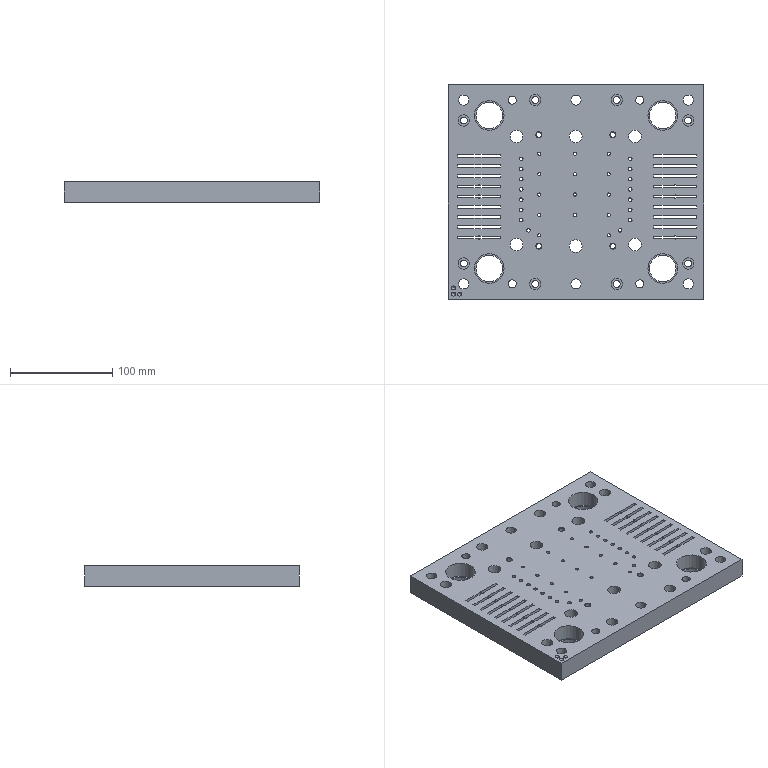Part | STEP file | 200 mesh_id2022 | 1 solid | 247 faces | box 250 x 210 x 20 mm | volume 913405 mm3 | plane 126 | cylinder 110 | cone 11 | commonest cylinder face diameters 3.2 x50 3.5 x16 6.8 x8 11 x8 10 x6 12.5 x6